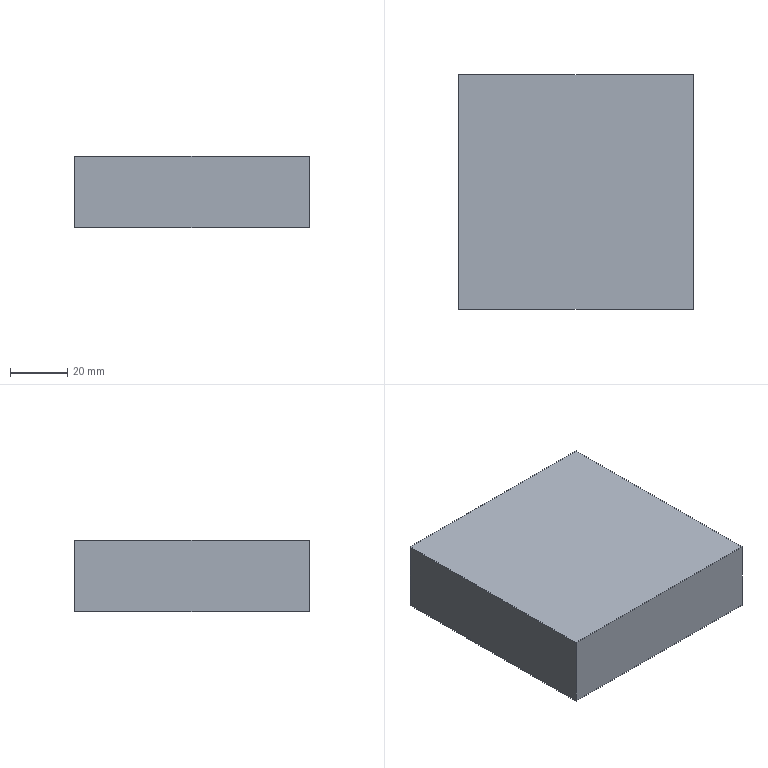Part | NX | features EXTRUDE 16, DATUM_CSYS 8, SKETCH 7, CHAMFER 5, BLEND 3, EXTRACT_STRING 2, DATUM_PLANE 1, HOLE PACKAGE 1, INTERSECTION_CURVES 1, Instance Feature 1, Mirror Feature 1, SIMPLE HOLE 1, SYMBOLIC_THREAD 1 | 2 solids | 124 faces | box 82 x 82 x 25 mm | volume 237764 mm3 | plane 78 | cylinder 40 | cone 6 | commonest cylinder face diameters 10 x20 2 x8 15 x3 13 x2 38 x2 56 x2